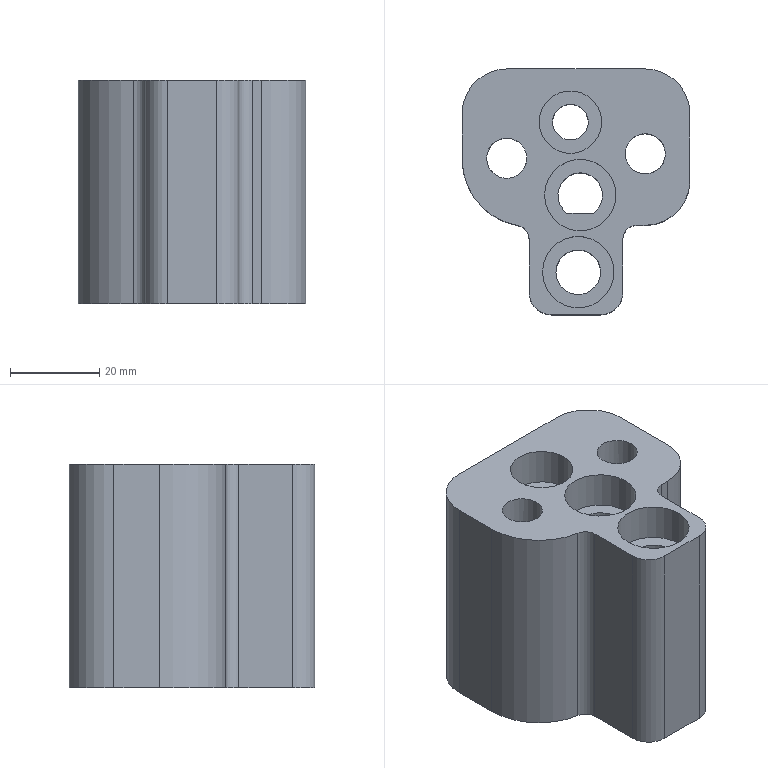Part | STEP file | PN_0023_id1002_x_t | 1 solid | 33 faces | box 51 x 55 x 50 mm | volume 79567 mm3 | cylinder 18 | plane 15 | commonest cylinder face diameters 10 x4 14 x3 20 x3 6 x2 9 x2 16 x2
STEP:
#1=CARTESIAN_POINT('',(276.,20.,95.));
#2=VERTEX_POINT('',#1);
#3=CARTESIAN_POINT('',(276.,8.,95.));
#4=VERTEX_POINT('',#3);
#5=CARTESIAN_POINT('',(276.,28.807,95.));
#6=DIRECTION('',(0.,-1.,0.));
#7=VECTOR('',#6,1.);
#8=LINE('',#5,#7);
#9=EDGE_CURVE('',#2,#4,#8,.T.);
#10=ORIENTED_EDGE('',*,*,#9,.T.);
#11=CARTESIAN_POINT('',(276.,8.,45.));
#12=VERTEX_POINT('',#11);
#13=CARTESIAN_POINT('',(276.,8.,95.));
#14=DIRECTION('',(0.,0.,-1.));
#15=VECTOR('',#14,1.);
#16=LINE('',#13,#15);
#17=EDGE_CURVE('',#4,#12,#16,.T.);
#18=ORIENTED_EDGE('',*,*,#17,.T.);
#19=CARTESIAN_POINT('',(276.,20.,45.));
#20=VERTEX_POINT('',#19);
#21=CARTESIAN_POINT('',(276.,28.807,45.));
#22=DIRECTION('',(0.,1.,0.));
#23=VECTOR('',#22,1.);
#24=LINE('',#21,#23);
#25=EDGE_CURVE('',#12,#20,#24,.T.);
#26=ORIENTED_EDGE('',*,*,#25,.T.);
#27=CARTESIAN_POINT('',(276.,20.,95.));
#28=DIRECTION('',(0.,0.,1.));
#29=VECTOR('',#28,1.);
#30=LINE('',#27,#29);
#31=EDGE_CURVE('',#20,#2,#30,.T.);
#32=ORIENTED_EDGE('',*,*,#31,.T.);
#33=EDGE_LOOP('',(#10,#18,#26,#32));
#34=FACE_OUTER_BOUND('',#33,.T.);
#35=CARTESIAN_POINT('',(276.,28.807,95.));
#36=DIRECTION('',(1.,0.,0.));
#37=DIRECTION('',(0.,0.,-1.));
#38=AXIS2_PLACEMENT_3D('',#35,#36,#37);
#39=PLANE('',#38);
#40=ADVANCED_FACE('',(#34),#39,.T.);
#41=CARTESIAN_POINT('',(255.,20.,45.));
#42=VERTEX_POINT('',#41);
#43=CARTESIAN_POINT('',(255.,8.,45.));
#44=VERTEX_POINT('',#43);
#45=CARTESIAN_POINT('',(255.,28.807,45.));
#46=DIRECTION('',(0.,-1.,0.));
#47=VECTOR('',#46,1.);
#48=LINE('',#45,#47);
#49=EDGE_CURVE('',#42,#44,#48,.T.);
#50=ORIENTED_EDGE('',*,*,#49,.T.);
#51=CARTESIAN_POINT('',(255.,8.,95.));
#52=VERTEX_POINT('',#51);
#53=CARTESIAN_POINT('',(255.,8.,95.));
#54=DIRECTION('',(0.,0.,1.));
#55=VECTOR('',#54,1.);
#56=LINE('',#53,#55);
#57=EDGE_CURVE('',#44,#52,#56,.T.);
#58=ORIENTED_EDGE('',*,*,#57,.T.);
#59=CARTESIAN_POINT('',(255.,20.,95.));
#60=VERTEX_POINT('',#59);
#61=CARTESIAN_POINT('',(255.,28.807,95.));
#62=DIRECTION('',(0.,1.,0.));
#63=VECTOR('',#62,1.);
#64=LINE('',#61,#63);
#65=EDGE_CURVE('',#52,#60,#64,.T.);
#66=ORIENTED_EDGE('',*,*,#65,.T.);
#67=CARTESIAN_POINT('',(255.,20.,95.));
#68=DIRECTION('',(0.,0.,-1.));
#69=VECTOR('',#68,1.);
#70=LINE('',#67,#69);
#71=EDGE_CURVE('',#60,#42,#70,.T.);
#72=ORIENTED_EDGE('',*,*,#71,.T.);
#73=EDGE_LOOP('',(#50,#58,#66,#72));
#74=FACE_OUTER_BOUND('',#73,.T.);
#75=CARTESIAN_POINT('',(255.,28.807,95.));
#76=DIRECTION('',(-1.,0.,0.));
#77=DIRECTION('',(0.,0.,1.));
#78=AXIS2_PLACEMENT_3D('',#75,#76,#77);
#79=PLANE('',#78);
#80=ADVANCED_FACE('',(#74),#79,.T.);
#81=CARTESIAN_POINT('',(263.45,25.762,45.));
#82=VERTEX_POINT('',#81);
#83=CARTESIAN_POINT('',(269.45,25.762,45.));
#84=VERTEX_POINT('',#83);
#85=CARTESIAN_POINT('',(266.45,25.762,45.));
#86=DIRECTION('',(1.,0.,0.));
#87=VECTOR('',#86,1.);
#88=LINE('',#85,#87);
#89=EDGE_CURVE('',#82,#84,#88,.T.);
#90=ORIENTED_EDGE('',*,*,#89,.T.);
#91=CARTESIAN_POINT('',(266.45,29.762,45.));
#92=DIRECTION('',(0.,0.,1.));
#93=DIRECTION('',(1.,0.,0.));
#94=AXIS2_PLACEMENT_3D('',#91,#92,#93);
#95=CIRCLE('',#94,5.);
#96=EDGE_CURVE('',#84,#82,#95,.T.);
#97=ORIENTED_EDGE('',*,*,#96,.T.);
#98=EDGE_LOOP('',(#90,#97));
#99=FACE_BOUND('',#98,.T.);
#100=CARTESIAN_POINT('',(271.,12.5,45.));
#101=VERTEX_POINT('',#100);
#102=CARTESIAN_POINT('',(266.,12.5,45.));
#103=DIRECTION('',(0.,0.,1.));
#104=DIRECTION('',(1.,0.,0.));
#105=AXIS2_PLACEMENT_3D('',#102,#103,#104);
#106=CIRCLE('',#105,5.);
#107=EDGE_CURVE('',#101,#101,#106,.T.);
#108=ORIENTED_EDGE('',*,*,#107,.T.);
#109=EDGE_LOOP('',(#108));
#110=FACE_BOUND('',#109,.T.);
#111=CARTESIAN_POINT('',(268.25,46.114,45.));
#112=VERTEX_POINT('',#111);
#113=CARTESIAN_POINT('',(264.25,46.114,45.));
#114=DIRECTION('',(0.,0.,1.));
#115=DIRECTION('',(1.,0.,0.));
#116=AXIS2_PLACEMENT_3D('',#113,#114,#115);
#117=CIRCLE('',#116,4.);
#118=EDGE_CURVE('',#112,#112,#117,.T.);
#119=ORIENTED_EDGE('',*,*,#118,.T.);
#120=EDGE_LOOP('',(#119));
#121=FACE_BOUND('',#120,.T.);
#122=CARTESIAN_POINT('',(281.,46.,45.));
#123=VERTEX_POINT('',#122);
#124=CARTESIAN_POINT('',(281.,39.,45.));
#125=DIRECTION('',(0.,0.,1.));
#126=DIRECTION('',(0.,1.,0.));
#127=AXIS2_PLACEMENT_3D('',#124,#125,#126);
#128=CIRCLE('',#127,7.);
#129=EDGE_CURVE('',#123,#123,#128,.T.);
#130=ORIENTED_EDGE('',*,*,#129,.T.);
#131=EDGE_LOOP('',(#130));
#132=FACE_BOUND('',#131,.T.);
#133=CARTESIAN_POINT('',(250.,31.,45.));
#134=VERTEX_POINT('',#133);
#135=CARTESIAN_POINT('',(250.,38.,45.));
#136=DIRECTION('',(0.,0.,1.));
#137=DIRECTION('',(0.,-1.,0.));
#138=AXIS2_PLACEMENT_3D('',#135,#136,#137);
#139=CIRCLE('',#138,7.);
#140=EDGE_CURVE('',#134,#134,#139,.T.);
#141=ORIENTED_EDGE('',*,*,#140,.T.);
#142=EDGE_LOOP('',(#141));
#143=FACE_BOUND('',#142,.T.);
#144=CARTESIAN_POINT('',(252.5,22.958,45.));
#145=VERTEX_POINT('',#144);
#146=CARTESIAN_POINT('',(252.,20.,45.));
#147=DIRECTION('',(0.,0.,1.));
#148=DIRECTION('',(1.,0.,0.));
#149=AXIS2_PLACEMENT_3D('',#146,#147,#148);
#150=CIRCLE('',#149,3.);
#151=EDGE_CURVE('',#42,#145,#150,.T.);
#152=ORIENTED_EDGE('',*,*,#151,.T.);
#153=CARTESIAN_POINT('',(240.,37.748,45.));
#154=VERTEX_POINT('',#153);
#155=CARTESIAN_POINT('',(255.,37.748,45.));
#156=DIRECTION('',(0.,0.,-1.));
#157=DIRECTION('',(1.,0.,0.));
#158=AXIS2_PLACEMENT_3D('',#155,#156,#157);
#159=CIRCLE('',#158,15.);
#160=EDGE_CURVE('',#145,#154,#159,.T.);
#161=ORIENTED_EDGE('',*,*,#160,.T.);
#162=CARTESIAN_POINT('',(240.,48.,45.));
#163=VERTEX_POINT('',#162);
#164=CARTESIAN_POINT('',(240.,28.807,45.));
#165=DIRECTION('',(0.,-1.,0.));
#166=VECTOR('',#165,1.);
#167=LINE('',#164,#166);
#168=EDGE_CURVE('',#163,#154,#167,.T.);
#169=ORIENTED_EDGE('',*,*,#168,.F.);
#170=CARTESIAN_POINT('',(250.,58.,45.));
#171=VERTEX_POINT('',#170);
#172=CARTESIAN_POINT('',(250.,48.,45.));
#173=DIRECTION('',(0.,0.,-1.));
#174=DIRECTION('',(1.,0.,0.));
#175=AXIS2_PLACEMENT_3D('',#172,#173,#174);
#176=CIRCLE('',#175,10.);
#177=EDGE_CURVE('',#163,#171,#176,.T.);
#178=ORIENTED_EDGE('',*,*,#177,.T.);
#179=CARTESIAN_POINT('',(281.,58.,45.));
#180=VERTEX_POINT('',#179);
#181=CARTESIAN_POINT('',(265.85,58.,45.));
#182=DIRECTION('',(-1.,0.,0.));
#183=VECTOR('',#182,1.);
#184=LINE('',#181,#183);
#185=EDGE_CURVE('',#180,#171,#184,.T.);
#186=ORIENTED_EDGE('',*,*,#185,.F.);
#187=CARTESIAN_POINT('',(291.,48.,45.));
#188=VERTEX_POINT('',#187);
#189=CARTESIAN_POINT('',(281.,48.,45.));
#190=DIRECTION('',(0.,0.,-1.));
#191=DIRECTION('',(1.,0.,0.));
#192=AXIS2_PLACEMENT_3D('',#189,#190,#191);
#193=CIRCLE('',#192,10.);
#194=EDGE_CURVE('',#180,#188,#193,.T.);
#195=ORIENTED_EDGE('',*,*,#194,.T.);
#196=CARTESIAN_POINT('',(291.,33.,45.));
#197=VERTEX_POINT('',#196);
#198=CARTESIAN_POINT('',(291.,58.,45.));
#199=DIRECTION('',(0.,-1.,0.));
#200=VECTOR('',#199,1.);
#201=LINE('',#198,#200);
#202=EDGE_CURVE('',#188,#197,#201,.T.);
#203=ORIENTED_EDGE('',*,*,#202,.T.);
#204=CARTESIAN_POINT('',(281.,23.,45.));
#205=VERTEX_POINT('',#204);
#206=CARTESIAN_POINT('',(281.,33.,45.));
#207=DIRECTION('',(0.,0.,-1.));
#208=DIRECTION('',(1.,0.,0.));
#209=AXIS2_PLACEMENT_3D('',#206,#207,#208);
#210=CIRCLE('',#209,10.);
#211=EDGE_CURVE('',#197,#205,#210,.T.);
#212=ORIENTED_EDGE('',*,*,#211,.T.);
#213=CARTESIAN_POINT('',(279.,23.,45.));
#214=VERTEX_POINT('',#213);
#215=CARTESIAN_POINT('',(265.85,23.,45.));
#216=DIRECTION('',(-1.,0.,0.));
#217=VECTOR('',#216,1.);
#218=LINE('',#215,#217);
#219=EDGE_CURVE('',#205,#214,#218,.T.);
#220=ORIENTED_EDGE('',*,*,#219,.T.);
#221=CARTESIAN_POINT('',(279.,20.,45.));
#222=DIRECTION('',(0.,0.,1.));
#223=DIRECTION('',(1.,0.,0.));
#224=AXIS2_PLACEMENT_3D('',#221,#222,#223);
#225=CIRCLE('',#224,3.);
#226=EDGE_CURVE('',#214,#20,#225,.T.);
#227=ORIENTED_EDGE('',*,*,#226,.T.);
#228=ORIENTED_EDGE('',*,*,#25,.F.);
#229=CARTESIAN_POINT('',(271.,3.,45.));
#230=VERTEX_POINT('',#229);
#231=CARTESIAN_POINT('',(271.,8.,45.));
#232=DIRECTION('',(0.,0.,-1.));
#233=DIRECTION('',(1.,0.,0.));
#234=AXIS2_PLACEMENT_3D('',#231,#232,#233);
#235=CIRCLE('',#234,5.);
#236=EDGE_CURVE('',#12,#230,#235,.T.);
#237=ORIENTED_EDGE('',*,*,#236,.T.);
#238=CARTESIAN_POINT('',(260.,3.,45.));
#239=VERTEX_POINT('',#238);
#240=CARTESIAN_POINT('',(265.85,3.,45.));
#241=DIRECTION('',(1.,0.,0.));
#242=VECTOR('',#241,1.);
#243=LINE('',#240,#242);
#244=EDGE_CURVE('',#239,#230,#243,.T.);
#245=ORIENTED_EDGE('',*,*,#244,.F.);
#246=CARTESIAN_POINT('',(260.,8.,45.));
#247=DIRECTION('',(0.,0.,-1.));
#248=DIRECTION('',(1.,0.,0.));
#249=AXIS2_PLACEMENT_3D('',#246,#247,#248);
#250=CIRCLE('',#249,5.);
#251=EDGE_CURVE('',#239,#44,#250,.T.);
#252=ORIENTED_EDGE('',*,*,#251,.T.);
#253=ORIENTED_EDGE('',*,*,#49,.F.);
#254=EDGE_LOOP('',(#152,#161,#169,#178,#186,#195,#203,#212,#220,#227,#228,#237,#245,#252,#253));
#255=FACE_BOUND('',#254,.T.);
#256=CARTESIAN_POINT('',(265.85,28.807,45.));
#257=DIRECTION('',(0.,0.,1.));
#258=DIRECTION('',(1.,0.,0.));
#259=AXIS2_PLACEMENT_3D('',#256,#257,#258);
#260=PLANE('',#259);
#261=ADVANCED_FACE('',(#99,#110,#121,#132,#143,#255),#260,.F.);
#262=ORIENTED_EDGE('',*,*,#244,.T.);
#263=CARTESIAN_POINT('',(271.,3.,95.));
#264=VERTEX_POINT('',#263);
#265=CARTESIAN_POINT('',(271.,3.,95.));
#266=DIRECTION('',(0.,0.,1.));
#267=VECTOR('',#266,1.);
#268=LINE('',#265,#267);
#269=EDGE_CURVE('',#230,#264,#268,.T.);
#270=ORIENTED_EDGE('',*,*,#269,.T.);
#271=CARTESIAN_POINT('',(260.,3.,95.));
#272=VERTEX_POINT('',#271);
#273=CARTESIAN_POINT('',(265.85,3.,95.));
#274=DIRECTION('',(-1.,0.,0.));
#275=VECTOR('',#274,1.);
#276=LINE('',#273,#275);
#277=EDGE_CURVE('',#264,#272,#276,.T.);
#278=ORIENTED_EDGE('',*,*,#277,.T.);
#279=CARTESIAN_POINT('',(260.,3.,95.));
#280=DIRECTION('',(0.,0.,-1.));
#281=VECTOR('',#280,1.);
#282=LINE('',#279,#281);
#283=EDGE_CURVE('',#272,#239,#282,.T.);
#284=ORIENTED_EDGE('',*,*,#283,.T.);
#285=EDGE_LOOP('',(#262,#270,#278,#284));
#286=FACE_OUTER_BOUND('',#285,.T.);
#287=CARTESIAN_POINT('',(265.85,3.,95.));
#288=DIRECTION('',(0.,-1.,0.));
#289=DIRECTION('',(0.,0.,-1.));
#290=AXIS2_PLACEMENT_3D('',#287,#288,#289);
#291=PLANE('',#290);
#292=ADVANCED_FACE('',(#286),#291,.T.);
#293=ORIENTED_EDGE('',*,*,#185,.T.);
#294=CARTESIAN_POINT('',(250.,58.,95.));
#295=VERTEX_POINT('',#294);
#296=CARTESIAN_POINT('',(250.,58.,95.));
#297=DIRECTION('',(0.,0.,1.));
#298=VECTOR('',#297,1.);
#299=LINE('',#296,#298);
#300=EDGE_CURVE('',#171,#295,#299,.T.);
#301=ORIENTED_EDGE('',*,*,#300,.T.);
#302=CARTESIAN_POINT('',(281.,58.,95.));
#303=VERTEX_POINT('',#302);
#304=CARTESIAN_POINT('',(265.85,58.,95.));
#305=DIRECTION('',(1.,0.,0.));
#306=VECTOR('',#305,1.);
#307=LINE('',#304,#306);
#308=EDGE_CURVE('',#295,#303,#307,.T.);
#309=ORIENTED_EDGE('',*,*,#308,.T.);
#310=CARTESIAN_POINT('',(281.,58.,45.));
#311=DIRECTION('',(0.,0.,-1.));
#312=VECTOR('',#311,1.);
#313=LINE('',#310,#312);
#314=EDGE_CURVE('',#303,#180,#313,.T.);
#315=ORIENTED_EDGE('',*,*,#314,.T.);
#316=EDGE_LOOP('',(#293,#301,#309,#315));
#317=FACE_OUTER_BOUND('',#316,.T.);
#318=CARTESIAN_POINT('',(265.85,58.,95.));
#319=DIRECTION('',(0.,1.,0.));
#320=DIRECTION('',(0.,0.,1.));
#321=AXIS2_PLACEMENT_3D('',#318,#319,#320);
#322=PLANE('',#321);
#323=ADVANCED_FACE('',(#317),#322,.T.);
#324=CARTESIAN_POINT('',(274.45,29.762,95.));
#325=VERTEX_POINT('',#324);
#326=CARTESIAN_POINT('',(266.45,29.762,95.));
#327=DIRECTION('',(0.,0.,-1.));
#328=DIRECTION('',(1.,0.,0.));
#329=AXIS2_PLACEMENT_3D('',#326,#327,#328);
#330=CIRCLE('',#329,8.);
#331=EDGE_CURVE('',#325,#325,#330,.T.);
#332=ORIENTED_EDGE('',*,*,#331,.T.);
#333=EDGE_LOOP('',(#332));
#334=FACE_BOUND('',#333,.T.);
#335=CARTESIAN_POINT('',(274.,12.5,95.));
#336=VERTEX_POINT('',#335);
#337=CARTESIAN_POINT('',(266.,12.5,95.));
#338=DIRECTION('',(0.,0.,-1.));
#339=DIRECTION('',(1.,0.,0.));
#340=AXIS2_PLACEMENT_3D('',#337,#338,#339);
#341=CIRCLE('',#340,8.);
#342=EDGE_CURVE('',#336,#336,#341,.T.);
#343=ORIENTED_EDGE('',*,*,#342,.T.);
#344=EDGE_LOOP('',(#343));
#345=FACE_BOUND('',#344,.T.);
#346=CARTESIAN_POINT('',(271.25,46.114,95.));
#347=VERTEX_POINT('',#346);
#348=CARTESIAN_POINT('',(264.25,46.114,95.));
#349=DIRECTION('',(0.,0.,-1.));
#350=DIRECTION('',(1.,0.,0.));
#351=AXIS2_PLACEMENT_3D('',#348,#349,#350);
#352=CIRCLE('',#351,7.);
#353=EDGE_CURVE('',#347,#347,#352,.T.);
#354=ORIENTED_EDGE('',*,*,#353,.T.);
#355=EDGE_LOOP('',(#354));
#356=FACE_BOUND('',#355,.T.);
#357=CARTESIAN_POINT('',(285.5,39.,95.));
#358=VERTEX_POINT('',#357);
#359=CARTESIAN_POINT('',(281.,39.,95.));
#360=DIRECTION('',(0.,0.,1.));
#361=DIRECTION('',(1.,0.,0.));
#362=AXIS2_PLACEMENT_3D('',#359,#360,#361);
#363=CIRCLE('',#362,4.5);
#364=EDGE_CURVE('',#358,#358,#363,.T.);
#365=ORIENTED_EDGE('',*,*,#364,.F.);
#366=EDGE_LOOP('',(#365));
#367=FACE_BOUND('',#366,.T.);
#368=CARTESIAN_POINT('',(254.5,38.,95.));
#369=VERTEX_POINT('',#368);
#370=CARTESIAN_POINT('',(250.,38.,95.));
#371=DIRECTION('',(0.,0.,1.));
#372=DIRECTION('',(1.,0.,0.));
#373=AXIS2_PLACEMENT_3D('',#370,#371,#372);
#374=CIRCLE('',#373,4.5);
#375=EDGE_CURVE('',#369,#369,#374,.T.);
#376=ORIENTED_EDGE('',*,*,#375,.F.);
#377=EDGE_LOOP('',(#376));
#378=FACE_BOUND('',#377,.T.);
#379=CARTESIAN_POINT('',(240.,48.,95.));
#380=VERTEX_POINT('',#379);
#381=CARTESIAN_POINT('',(240.,37.748,95.));
#382=VERTEX_POINT('',#381);
#383=CARTESIAN_POINT('',(240.,58.,95.));
#384=DIRECTION('',(0.,-1.,0.));
#385=VECTOR('',#384,1.);
#386=LINE('',#383,#385);
#387=EDGE_CURVE('',#380,#382,#386,.T.);
#388=ORIENTED_EDGE('',*,*,#387,.T.);
#389=CARTESIAN_POINT('',(252.5,22.958,95.));
#390=VERTEX_POINT('',#389);
#391=CARTESIAN_POINT('',(255.,37.748,95.));
#392=DIRECTION('',(0.,0.,1.));
#393=DIRECTION('',(1.,0.,0.));
#394=AXIS2_PLACEMENT_3D('',#391,#392,#393);
#395=CIRCLE('',#394,15.);
#396=EDGE_CURVE('',#382,#390,#395,.T.);
#397=ORIENTED_EDGE('',*,*,#396,.T.);
#398=CARTESIAN_POINT('',(252.,20.,95.));
#399=DIRECTION('',(0.,0.,-1.));
#400=DIRECTION('',(1.,0.,0.));
#401=AXIS2_PLACEMENT_3D('',#398,#399,#400);
#402=CIRCLE('',#401,3.);
#403=EDGE_CURVE('',#390,#60,#402,.T.);
#404=ORIENTED_EDGE('',*,*,#403,.T.);
#405=ORIENTED_EDGE('',*,*,#65,.F.);
#406=CARTESIAN_POINT('',(260.,8.,95.));
#407=DIRECTION('',(0.,0.,1.));
#408=DIRECTION('',(1.,0.,0.));
#409=AXIS2_PLACEMENT_3D('',#406,#407,#408);
#410=CIRCLE('',#409,5.);
#411=EDGE_CURVE('',#52,#272,#410,.T.);
#412=ORIENTED_EDGE('',*,*,#411,.T.);
#413=ORIENTED_EDGE('',*,*,#277,.F.);
#414=CARTESIAN_POINT('',(271.,8.,95.));
#415=DIRECTION('',(0.,0.,1.));
#416=DIRECTION('',(1.,0.,0.));
#417=AXIS2_PLACEMENT_3D('',#414,#415,#416);
#418=CIRCLE('',#417,5.);
#419=EDGE_CURVE('',#264,#4,#418,.T.);
#420=ORIENTED_EDGE('',*,*,#419,.T.);
#421=ORIENTED_EDGE('',*,*,#9,.F.);
#422=CARTESIAN_POINT('',(279.,23.,95.));
#423=VERTEX_POINT('',#422);
#424=CARTESIAN_POINT('',(279.,20.,95.));
#425=DIRECTION('',(0.,0.,-1.));
#426=DIRECTION('',(1.,0.,0.));
#427=AXIS2_PLACEMENT_3D('',#424,#425,#426);
#428=CIRCLE('',#427,3.);
#429=EDGE_CURVE('',#2,#423,#428,.T.);
#430=ORIENTED_EDGE('',*,*,#429,.T.);
#431=CARTESIAN_POINT('',(281.,23.,95.));
#432=VERTEX_POINT('',#431);
#433=CARTESIAN_POINT('',(265.85,23.,95.));
#434=DIRECTION('',(1.,0.,0.));
#435=VECTOR('',#434,1.);
#436=LINE('',#433,#435);
#437=EDGE_CURVE('',#423,#432,#436,.T.);
#438=ORIENTED_EDGE('',*,*,#437,.T.);
#439=CARTESIAN_POINT('',(291.,33.,95.));
#440=VERTEX_POINT('',#439);
#441=CARTESIAN_POINT('',(281.,33.,95.));
#442=DIRECTION('',(0.,0.,1.));
#443=DIRECTION('',(1.,0.,0.));
#444=AXIS2_PLACEMENT_3D('',#441,#442,#443);
#445=CIRCLE('',#444,10.);
#446=EDGE_CURVE('',#432,#440,#445,.T.);
#447=ORIENTED_EDGE('',*,*,#446,.T.);
#448=CARTESIAN_POINT('',(291.,48.,95.));
#449=VERTEX_POINT('',#448);
#450=CARTESIAN_POINT('',(291.,28.807,95.));
#451=DIRECTION('',(0.,-1.,0.));
#452=VECTOR('',#451,1.);
#453=LINE('',#450,#452);
#454=EDGE_CURVE('',#449,#440,#453,.T.);
#455=ORIENTED_EDGE('',*,*,#454,.F.);
#456=CARTESIAN_POINT('',(281.,48.,95.));
#457=DIRECTION('',(0.,0.,1.));
#458=DIRECTION('',(1.,0.,0.));
#459=AXIS2_PLACEMENT_3D('',#456,#457,#458);
#460=CIRCLE('',#459,10.);
#461=EDGE_CURVE('',#449,#303,#460,.T.);
#462=ORIENTED_EDGE('',*,*,#461,.T.);
#463=ORIENTED_EDGE('',*,*,#308,.F.);
#464=CARTESIAN_POINT('',(250.,48.,95.));
#465=DIRECTION('',(0.,0.,1.));
#466=DIRECTION('',(1.,0.,0.));
#467=AXIS2_PLACEMENT_3D('',#464,#465,#466);
#468=CIRCLE('',#467,10.);
#469=EDGE_CURVE('',#295,#380,#468,.T.);
#470=ORIENTED_EDGE('',*,*,#469,.T.);
#471=EDGE_LOOP('',(#388,#397,#404,#405,#412,#413,#420,#421,#430,#438,#447,#455,#462,#463,#470));
#472=FACE_BOUND('',#471,.T.);
#473=CARTESIAN_POINT('',(265.85,28.807,95.));
#474=DIRECTION('',(0.,0.,1.));
#475=DIRECTION('',(1.,0.,0.));
#476=AXIS2_PLACEMENT_3D('',#473,#474,#475);
#477=PLANE('',#476);
#478=ADVANCED_FACE('',(#334,#345,#356,#367,#378,#472),#477,.T.);
#479=ORIENTED_EDGE('',*,*,#168,.T.);
#480=CARTESIAN_POINT('',(240.,37.748,95.));
#481=DIRECTION('',(0.,0.,1.));
#482=VECTOR('',#481,1.);
#483=LINE('',#480,#482);
#484=EDGE_CURVE('',#154,#382,#483,.T.);
#485=ORIENTED_EDGE('',*,*,#484,.T.);
#486=ORIENTED_EDGE('',*,*,#387,.F.);
#487=CARTESIAN_POINT('',(240.,48.,45.));
#488=DIRECTION('',(0.,0.,-1.));
#489=VECTOR('',#488,1.);
#490=LINE('',#487,#489);
#491=EDGE_CURVE('',#380,#163,#490,.T.);
#492=ORIENTED_EDGE('',*,*,#491,.T.);
#493=EDGE_LOOP('',(#479,#485,#486,#492));
#494=FACE_OUTER_BOUND('',#493,.T.);
#495=CARTESIAN_POINT('',(240.,58.,95.));
#496=DIRECTION('',(1.,0.,0.));
#497=DIRECTION('',(0.,0.,-1.));
#498=AXIS2_PLACEMENT_3D('',#495,#496,#497);
#499=PLANE('',#498);
#500=ADVANCED_FACE('',(#494),#499,.F.);
#501=ORIENTED_EDGE('',*,*,#219,.F.);
#502=CARTESIAN_POINT('',(281.,23.,95.));
#503=DIRECTION('',(0.,0.,1.));
#504=VECTOR('',#503,1.);
#505=LINE('',#502,#504);
#506=EDGE_CURVE('',#205,#432,#505,.T.);
#507=ORIENTED_EDGE('',*,*,#506,.T.);
#508=ORIENTED_EDGE('',*,*,#437,.F.);
#509=CARTESIAN_POINT('',(279.,23.,95.));
#510=DIRECTION('',(0.,0.,-1.));
#511=VECTOR('',#510,1.);
#512=LINE('',#509,#511);
#513=EDGE_CURVE('',#423,#214,#512,.T.);
#514=ORIENTED_EDGE('',*,*,#513,.T.);
#515=EDGE_LOOP('',(#501,#507,#508,#514));
#516=FACE_OUTER_BOUND('',#515,.T.);
#517=CARTESIAN_POINT('',(265.85,23.,95.));
#518=DIRECTION('',(0.,1.,0.));
#519=DIRECTION('',(0.,0.,1.));
#520=AXIS2_PLACEMENT_3D('',#517,#518,#519);
#521=PLANE('',#520);
#522=ADVANCED_FACE('',(#516),#521,.F.);
#523=ORIENTED_EDGE('',*,*,#454,.T.);
#524=CARTESIAN_POINT('',(291.,33.,95.));
#525=DIRECTION('',(0.,0.,-1.));
#526=VECTOR('',#525,1.);
#527=LINE('',#524,#526);
#528=EDGE_CURVE('',#440,#197,#527,.T.);
#529=ORIENTED_EDGE('',*,*,#528,.T.);
#530=ORIENTED_EDGE('',*,*,#202,.F.);
#531=CARTESIAN_POINT('',(291.,48.,95.));
#532=DIRECTION('',(0.,0.,1.));
#533=VECTOR('',#532,1.);
#534=LINE('',#531,#533);
#535=EDGE_CURVE('',#188,#449,#534,.T.);
#536=ORIENTED_EDGE('',*,*,#535,.T.);
#537=EDGE_LOOP('',(#523,#529,#530,#536));
#538=FACE_OUTER_BOUND('',#537,.T.);
#539=CARTESIAN_POINT('',(291.,58.,95.));
#540=DIRECTION('',(1.,0.,0.));
#541=DIRECTION('',(0.,0.,-1.));
#542=AXIS2_PLACEMENT_3D('',#539,#540,#541);
#543=PLANE('',#542);
#544=ADVANCED_FACE('',(#538),#543,.T.);
#545=ORIENTED_EDGE('',*,*,#226,.F.);
#546=ORIENTED_EDGE('',*,*,#513,.F.);
#547=ORIENTED_EDGE('',*,*,#429,.F.);
#548=ORIENTED_EDGE('',*,*,#31,.F.);
#549=EDGE_LOOP('',(#545,#546,#547,#548));
#550=FACE_OUTER_BOUND('',#549,.T.);
#551=CARTESIAN_POINT('',(279.,20.,95.));
#552=DIRECTION('',(0.,0.,1.));
#553=DIRECTION('',(1.,0.,0.));
#554=AXIS2_PLACEMENT_3D('',#551,#552,#553);
#555=CYLINDRICAL_SURFACE('',#554,3.);
#556=ADVANCED_FACE('',(#550),#555,.F.);
#557=ORIENTED_EDGE('',*,*,#403,.F.);
#558=CARTESIAN_POINT('',(252.5,22.958,70.));
#559=DIRECTION('',(0.,0.,-1.));
#560=VECTOR('',#559,1.);
#561=LINE('',#558,#560);
#562=EDGE_CURVE('',#390,#145,#561,.T.);
#563=ORIENTED_EDGE('',*,*,#562,.T.);
#564=ORIENTED_EDGE('',*,*,#151,.F.);
#565=ORIENTED_EDGE('',*,*,#71,.F.);
#566=EDGE_LOOP('',(#557,#563,#564,#565));
#567=FACE_OUTER_BOUND('',#566,.T.);
#568=CARTESIAN_POINT('',(252.,20.,95.));
#569=DIRECTION('',(0.,0.,-1.));
#570=DIRECTION('',(-1.,0.,0.));
#571=AXIS2_PLACEMENT_3D('',#568,#569,#570);
#572=CYLINDRICAL_SURFACE('',#571,3.);
#573=ADVANCED_FACE('',(#567),#572,.F.);
#574=ORIENTED_EDGE('',*,*,#446,.F.);
#575=ORIENTED_EDGE('',*,*,#506,.F.);
#576=ORIENTED_EDGE('',*,*,#211,.F.);
#577=ORIENTED_EDGE('',*,*,#528,.F.);
#578=EDGE_LOOP('',(#574,#575,#576,#577));
#579=FACE_OUTER_BOUND('',#578,.T.);
#580=CARTESIAN_POINT('',(281.,33.,95.));
#581=DIRECTION('',(0.,0.,1.));
#582=DIRECTION('',(1.,0.,0.));
#583=AXIS2_PLACEMENT_3D('',#580,#581,#582);
#584=CYLINDRICAL_SURFACE('',#583,10.);
#585=ADVANCED_FACE('',(#579),#584,.T.);
#586=ORIENTED_EDGE('',*,*,#469,.F.);
#587=ORIENTED_EDGE('',*,*,#300,.F.);
#588=ORIENTED_EDGE('',*,*,#177,.F.);
#589=ORIENTED_EDGE('',*,*,#491,.F.);
#590=EDGE_LOOP('',(#586,#587,#588,#589));
#591=FACE_OUTER_BOUND('',#590,.T.);
#592=CARTESIAN_POINT('',(250.,48.,95.));
#593=DIRECTION('',(0.,0.,1.));
#594=DIRECTION('',(1.,0.,0.));
#595=AXIS2_PLACEMENT_3D('',#592,#593,#594);
#596=CYLINDRICAL_SURFACE('',#595,10.);
#597=ADVANCED_FACE('',(#591),#596,.T.);
#598=ORIENTED_EDGE('',*,*,#461,.F.);
#599=ORIENTED_EDGE('',*,*,#535,.F.);
#600=ORIENTED_EDGE('',*,*,#194,.F.);
#601=ORIENTED_EDGE('',*,*,#314,.F.);
#602=EDGE_LOOP('',(#598,#599,#600,#601));
#603=FACE_OUTER_BOUND('',#602,.T.);
#604=CARTESIAN_POINT('',(281.,48.,95.));
#605=DIRECTION('',(0.,0.,-1.));
#606=DIRECTION('',(-1.,0.,0.));
#607=AXIS2_PLACEMENT_3D('',#604,#605,#606);
#608=CYLINDRICAL_SURFACE('',#607,10.);
#609=ADVANCED_FACE('',(#603),#608,.T.);
#610=ORIENTED_EDGE('',*,*,#419,.F.);
#611=ORIENTED_EDGE('',*,*,#269,.F.);
#612=ORIENTED_EDGE('',*,*,#236,.F.);
#613=ORIENTED_EDGE('',*,*,#17,.F.);
#614=EDGE_LOOP('',(#610,#611,#612,#613));
#615=FACE_OUTER_BOUND('',#614,.T.);
#616=CARTESIAN_POINT('',(271.,8.,95.));
#617=DIRECTION('',(0.,0.,-1.));
#618=DIRECTION('',(-1.,0.,0.));
#619=AXIS2_PLACEMENT_3D('',#616,#617,#618);
#620=CYLINDRICAL_SURFACE('',#619,5.);
#621=ADVANCED_FACE('',(#615),#620,.T.);
#622=ORIENTED_EDGE('',*,*,#411,.F.);
#623=ORIENTED_EDGE('',*,*,#57,.F.);
#624=ORIENTED_EDGE('',*,*,#251,.F.);
#625=ORIENTED_EDGE('',*,*,#283,.F.);
#626=EDGE_LOOP('',(#622,#623,#624,#625));
#627=FACE_OUTER_BOUND('',#626,.T.);
#628=CARTESIAN_POINT('',(260.,8.,95.));
#629=DIRECTION('',(0.,0.,-1.));
#630=DIRECTION('',(-1.,0.,0.));
#631=AXIS2_PLACEMENT_3D('',#628,#629,#630);
#632=CYLINDRICAL_SURFACE('',#631,5.);
#633=ADVANCED_FACE('',(#627),#632,.T.);
#634=ORIENTED_EDGE('',*,*,#396,.F.);
#635=ORIENTED_EDGE('',*,*,#484,.F.);
#636=ORIENTED_EDGE('',*,*,#160,.F.);
#637=ORIENTED_EDGE('',*,*,#562,.F.);
#638=EDGE_LOOP('',(#634,#635,#636,#637));
#639=FACE_OUTER_BOUND('',#638,.T.);
#640=CARTESIAN_POINT('',(255.,37.748,95.));
#641=DIRECTION('',(0.,0.,-1.));
#642=DIRECTION('',(-1.,0.,0.));
#643=AXIS2_PLACEMENT_3D('',#640,#641,#642);
#644=CYLINDRICAL_SURFACE('',#643,15.);
#645=ADVANCED_FACE('',(#639),#644,.T.);
#646=ORIENTED_EDGE('',*,*,#375,.T.);
#647=EDGE_LOOP('',(#646));
#648=FACE_BOUND('',#647,.T.);
#649=CARTESIAN_POINT('',(250.,33.5,75.));
#650=VERTEX_POINT('',#649);
#651=CARTESIAN_POINT('',(250.,38.,75.));
#652=DIRECTION('',(0.,0.,1.));
#653=DIRECTION('',(0.,-1.,0.));
#654=AXIS2_PLACEMENT_3D('',#651,#652,#653);
#655=CIRCLE('',#654,4.5);
#656=EDGE_CURVE('',#650,#650,#655,.T.);
#657=ORIENTED_EDGE('',*,*,#656,.F.);
#658=EDGE_LOOP('',(#657));
#659=FACE_BOUND('',#658,.T.);
#660=CARTESIAN_POINT('',(250.,38.,105.));
#661=DIRECTION('',(0.,0.,-1.));
#662=DIRECTION('',(0.,1.,0.));
#663=AXIS2_PLACEMENT_3D('',#660,#661,#662);
#664=CYLINDRICAL_SURFACE('',#663,4.5);
#665=ADVANCED_FACE('',(#648,#659),#664,.F.);
#666=ORIENTED_EDGE('',*,*,#656,.T.);
#667=EDGE_LOOP('',(#666));
#668=FACE_BOUND('',#667,.T.);
#669=CARTESIAN_POINT('',(250.,45.,75.));
#670=VERTEX_POINT('',#669);
#671=CARTESIAN_POINT('',(250.,38.,75.));
#672=DIRECTION('',(0.,0.,1.));
#673=DIRECTION('',(0.,1.,0.));
#674=AXIS2_PLACEMENT_3D('',#671,#672,#673);
#675=CIRCLE('',#674,7.);
#676=EDGE_CURVE('',#670,#670,#675,.T.);
#677=ORIENTED_EDGE('',*,*,#676,.F.);
#678=EDGE_LOOP('',(#677));
#679=FACE_BOUND('',#678,.T.);
#680=CARTESIAN_POINT('',(250.,38.,75.));
#681=DIRECTION('',(0.,0.,1.));
#682=DIRECTION('',(0.,-1.,0.));
#683=AXIS2_PLACEMENT_3D('',#680,#681,#682);
#684=PLANE('',#683);
#685=ADVANCED_FACE('',(#668,#679),#684,.F.);
#686=ORIENTED_EDGE('',*,*,#140,.F.);
#687=EDGE_LOOP('',(#686));
#688=FACE_BOUND('',#687,.T.);
#689=ORIENTED_EDGE('',*,*,#676,.T.);
#690=EDGE_LOOP('',(#689));
#691=FACE_BOUND('',#690,.T.);
#692=CARTESIAN_POINT('',(250.,38.,75.));
#693=DIRECTION('',(0.,0.,-1.));
#694=DIRECTION('',(0.,1.,0.));
#695=AXIS2_PLACEMENT_3D('',#692,#693,#694);
#696=CYLINDRICAL_SURFACE('',#695,7.);
#697=ADVANCED_FACE('',(#688,#691),#696,.F.);
#698=ORIENTED_EDGE('',*,*,#364,.T.);
#699=EDGE_LOOP('',(#698));
#700=FACE_BOUND('',#699,.T.);
#701=CARTESIAN_POINT('',(281.,43.5,75.));
#702=VERTEX_POINT('',#701);
#703=CARTESIAN_POINT('',(281.,39.,75.));
#704=DIRECTION('',(0.,0.,1.));
#705=DIRECTION('',(0.,1.,0.));
#706=AXIS2_PLACEMENT_3D('',#703,#704,#705);
#707=CIRCLE('',#706,4.5);
#708=EDGE_CURVE('',#702,#702,#707,.T.);
#709=ORIENTED_EDGE('',*,*,#708,.F.);
#710=EDGE_LOOP('',(#709));
#711=FACE_BOUND('',#710,.T.);
#712=CARTESIAN_POINT('',(281.,39.,105.));
#713=DIRECTION('',(0.,0.,-1.));
#714=DIRECTION('',(0.,-1.,0.));
#715=AXIS2_PLACEMENT_3D('',#712,#713,#714);
#716=CYLINDRICAL_SURFACE('',#715,4.5);
#717=ADVANCED_FACE('',(#700,#711),#716,.F.);
#718=ORIENTED_EDGE('',*,*,#708,.T.);
#719=EDGE_LOOP('',(#718));
#720=FACE_BOUND('',#719,.T.);
#721=CARTESIAN_POINT('',(281.,32.,75.));
#722=VERTEX_POINT('',#721);
#723=CARTESIAN_POINT('',(281.,39.,75.));
#724=DIRECTION('',(0.,0.,1.));
#725=DIRECTION('',(0.,-1.,0.));
#726=AXIS2_PLACEMENT_3D('',#723,#724,#725);
#727=CIRCLE('',#726,7.);
#728=EDGE_CURVE('',#722,#722,#727,.T.);
#729=ORIENTED_EDGE('',*,*,#728,.F.);
#730=EDGE_LOOP('',(#729));
#731=FACE_BOUND('',#730,.T.);
#732=CARTESIAN_POINT('',(281.,39.,75.));
#733=DIRECTION('',(0.,0.,1.));
#734=DIRECTION('',(0.,1.,0.));
#735=AXIS2_PLACEMENT_3D('',#732,#733,#734);
#736=PLANE('',#735);
#737=ADVANCED_FACE('',(#720,#731),#736,.F.);
#738=ORIENTED_EDGE('',*,*,#129,.F.);
#739=EDGE_LOOP('',(#738));
#740=FACE_BOUND('',#739,.T.);
#741=ORIENTED_EDGE('',*,*,#728,.T.);
#742=EDGE_LOOP('',(#741));
#743=FACE_BOUND('',#742,.T.);
#744=CARTESIAN_POINT('',(281.,39.,75.));
#745=DIRECTION('',(0.,0.,-1.));
#746=DIRECTION('',(0.,-1.,0.));
#747=AXIS2_PLACEMENT_3D('',#744,#745,#746);
#748=CYLINDRICAL_SURFACE('',#747,7.);
#749=ADVANCED_FACE('',(#740,#743),#748,.F.);
#750=CARTESIAN_POINT('',(260.25,46.114,86.7));
#751=VERTEX_POINT('',#750);
#752=CARTESIAN_POINT('',(264.25,46.114,86.7));
#753=DIRECTION('',(0.,0.,1.));
#754=DIRECTION('',(-1.,0.,0.));
#755=AXIS2_PLACEMENT_3D('',#752,#753,#754);
#756=CIRCLE('',#755,4.);
#757=EDGE_CURVE('',#751,#751,#756,.T.);
#758=ORIENTED_EDGE('',*,*,#757,.F.);
#759=EDGE_LOOP('',(#758));
#760=FACE_BOUND('',#759,.T.);
#761=CARTESIAN_POINT('',(257.25,46.114,86.7));
#762=VERTEX_POINT('',#761);
#763=CARTESIAN_POINT('',(264.25,46.114,86.7));
#764=DIRECTION('',(0.,0.,-1.));
#765=DIRECTION('',(-1.,0.,0.));
#766=AXIS2_PLACEMENT_3D('',#763,#764,#765);
#767=CIRCLE('',#766,7.);
#768=EDGE_CURVE('',#762,#762,#767,.T.);
#769=ORIENTED_EDGE('',*,*,#768,.F.);
#770=EDGE_LOOP('',(#769));
#771=FACE_BOUND('',#770,.T.);
#772=CARTESIAN_POINT('',(264.25,46.114,86.7));
#773=DIRECTION('',(0.,0.,-1.));
#774=DIRECTION('',(-1.,0.,0.));
#775=AXIS2_PLACEMENT_3D('',#772,#773,#774);
#776=PLANE('',#775);
#777=ADVANCED_FACE('',(#760,#771),#776,.F.);
#778=ORIENTED_EDGE('',*,*,#768,.T.);
#779=EDGE_LOOP('',(#778));
#780=FACE_BOUND('',#779,.T.);
#781=ORIENTED_EDGE('',*,*,#353,.F.);
#782=EDGE_LOOP('',(#781));
#783=FACE_BOUND('',#782,.T.);
#784=CARTESIAN_POINT('',(264.25,46.114,94.559));
#785=DIRECTION('',(0.,0.,-1.));
#786=DIRECTION('',(0.,-1.,0.));
#787=AXIS2_PLACEMENT_3D('',#784,#785,#786);
#788=CYLINDRICAL_SURFACE('',#787,7.);
#789=ADVANCED_FACE('',(#780,#783),#788,.F.);
#790=ORIENTED_EDGE('',*,*,#757,.T.);
#791=EDGE_LOOP('',(#790));
#792=FACE_BOUND('',#791,.T.);
#793=ORIENTED_EDGE('',*,*,#118,.F.);
#794=EDGE_LOOP('',(#793));
#795=FACE_BOUND('',#794,.T.);
#796=CARTESIAN_POINT('',(264.25,46.114,85.5));
#797=DIRECTION('',(0.,0.,-1.));
#798=DIRECTION('',(0.,-1.,0.));
#799=AXIS2_PLACEMENT_3D('',#796,#797,#798);
#800=CYLINDRICAL_SURFACE('',#799,4.);
#801=ADVANCED_FACE('',(#792,#795),#800,.F.);
#802=CARTESIAN_POINT('',(261.,12.5,86.7));
#803=VERTEX_POINT('',#802);
#804=CARTESIAN_POINT('',(266.,12.5,86.7));
#805=DIRECTION('',(0.,0.,1.));
#806=DIRECTION('',(-1.,0.,0.));
#807=AXIS2_PLACEMENT_3D('',#804,#805,#806);
#808=CIRCLE('',#807,5.);
#809=EDGE_CURVE('',#803,#803,#808,.T.);
#810=ORIENTED_EDGE('',*,*,#809,.F.);
#811=EDGE_LOOP('',(#810));
#812=FACE_BOUND('',#811,.T.);
#813=CARTESIAN_POINT('',(258.,12.5,86.7));
#814=VERTEX_POINT('',#813);
#815=CARTESIAN_POINT('',(266.,12.5,86.7));
#816=DIRECTION('',(0.,0.,-1.));
#817=DIRECTION('',(-1.,0.,0.));
#818=AXIS2_PLACEMENT_3D('',#815,#816,#817);
#819=CIRCLE('',#818,8.);
#820=EDGE_CURVE('',#814,#814,#819,.T.);
#821=ORIENTED_EDGE('',*,*,#820,.F.);
#822=EDGE_LOOP('',(#821));
#823=FACE_BOUND('',#822,.T.);
#824=CARTESIAN_POINT('',(266.,12.5,86.7));
#825=DIRECTION('',(0.,0.,-1.));
#826=DIRECTION('',(-1.,0.,0.));
#827=AXIS2_PLACEMENT_3D('',#824,#825,#826);
#828=PLANE('',#827);
#829=ADVANCED_FACE('',(#812,#823),#828,.F.);
#830=ORIENTED_EDGE('',*,*,#820,.T.);
#831=EDGE_LOOP('',(#830));
#832=FACE_BOUND('',#831,.T.);
#833=ORIENTED_EDGE('',*,*,#342,.F.);
#834=EDGE_LOOP('',(#833));
#835=FACE_BOUND('',#834,.T.);
#836=CARTESIAN_POINT('',(266.,12.5,94.559));
#837=DIRECTION('',(0.,0.,-1.));
#838=DIRECTION('',(0.,-1.,0.));
#839=AXIS2_PLACEMENT_3D('',#836,#837,#838);
#840=CYLINDRICAL_SURFACE('',#839,8.);
#841=ADVANCED_FACE('',(#832,#835),#840,.F.);
#842=ORIENTED_EDGE('',*,*,#809,.T.);
#843=EDGE_LOOP('',(#842));
#844=FACE_BOUND('',#843,.T.);
#845=ORIENTED_EDGE('',*,*,#107,.F.);
#846=EDGE_LOOP('',(#845));
#847=FACE_BOUND('',#846,.T.);
#848=CARTESIAN_POINT('',(266.,12.5,85.5));
#849=DIRECTION('',(0.,0.,-1.));
#850=DIRECTION('',(0.,-1.,0.));
#851=AXIS2_PLACEMENT_3D('',#848,#849,#850);
#852=CYLINDRICAL_SURFACE('',#851,5.);
#853=ADVANCED_FACE('',(#844,#847),#852,.F.);
#854=CARTESIAN_POINT('',(269.45,25.762,86.7));
#855=VERTEX_POINT('',#854);
#856=CARTESIAN_POINT('',(263.45,25.762,86.7));
#857=VERTEX_POINT('',#856);
#858=CARTESIAN_POINT('',(266.45,25.762,86.7));
#859=DIRECTION('',(-1.,0.,0.));
#860=VECTOR('',#859,1.);
#861=LINE('',#858,#860);
#862=EDGE_CURVE('',#855,#857,#861,.T.);
#863=ORIENTED_EDGE('',*,*,#862,.T.);
#864=CARTESIAN_POINT('',(266.45,29.762,86.7));
#865=DIRECTION('',(0.,0.,1.));
#866=DIRECTION('',(-1.,0.,0.));
#867=AXIS2_PLACEMENT_3D('',#864,#865,#866);
#868=CIRCLE('',#867,5.);
#869=EDGE_CURVE('',#855,#857,#868,.T.);
#870=ORIENTED_EDGE('',*,*,#869,.F.);
#871=EDGE_LOOP('',(#863,#870));
#872=FACE_BOUND('',#871,.T.);
#873=CARTESIAN_POINT('',(258.45,29.762,86.7));
#874=VERTEX_POINT('',#873);
#875=CARTESIAN_POINT('',(266.45,29.762,86.7));
#876=DIRECTION('',(0.,0.,-1.));
#877=DIRECTION('',(-1.,0.,0.));
#878=AXIS2_PLACEMENT_3D('',#875,#876,#877);
#879=CIRCLE('',#878,8.);
#880=EDGE_CURVE('',#874,#874,#879,.T.);
#881=ORIENTED_EDGE('',*,*,#880,.F.);
#882=EDGE_LOOP('',(#881));
#883=FACE_BOUND('',#882,.T.);
#884=CARTESIAN_POINT('',(266.45,29.762,86.7));
#885=DIRECTION('',(0.,0.,-1.));
#886=DIRECTION('',(-1.,0.,0.));
#887=AXIS2_PLACEMENT_3D('',#884,#885,#886);
#888=PLANE('',#887);
#889=ADVANCED_FACE('',(#872,#883),#888,.F.);
#890=ORIENTED_EDGE('',*,*,#880,.T.);
#891=EDGE_LOOP('',(#890));
#892=FACE_BOUND('',#891,.T.);
#893=ORIENTED_EDGE('',*,*,#331,.F.);
#894=EDGE_LOOP('',(#893));
#895=FACE_BOUND('',#894,.T.);
#896=CARTESIAN_POINT('',(266.45,29.762,94.559));
#897=DIRECTION('',(0.,0.,-1.));
#898=DIRECTION('',(0.,-1.,0.));
#899=AXIS2_PLACEMENT_3D('',#896,#897,#898);
#900=CYLINDRICAL_SURFACE('',#899,8.);
#901=ADVANCED_FACE('',(#892,#895),#900,.F.);
#902=CARTESIAN_POINT('',(269.45,25.762,85.5));
#903=DIRECTION('',(0.,0.,1.));
#904=VECTOR('',#903,1.);
#905=LINE('',#902,#904);
#906=EDGE_CURVE('',#84,#855,#905,.T.);
#907=ORIENTED_EDGE('',*,*,#906,.F.);
#908=ORIENTED_EDGE('',*,*,#89,.F.);
#909=CARTESIAN_POINT('',(263.45,25.762,85.5));
#910=DIRECTION('',(0.,0.,-1.));
#911=VECTOR('',#910,1.);
#912=LINE('',#909,#911);
#913=EDGE_CURVE('',#857,#82,#912,.T.);
#914=ORIENTED_EDGE('',*,*,#913,.F.);
#915=ORIENTED_EDGE('',*,*,#862,.F.);
#916=EDGE_LOOP('',(#907,#908,#914,#915));
#917=FACE_OUTER_BOUND('',#916,.T.);
#918=CARTESIAN_POINT('',(266.45,25.762,56.595));
#919=DIRECTION('',(0.,-1.,0.));
#920=DIRECTION('',(0.,0.,-1.));
#921=AXIS2_PLACEMENT_3D('',#918,#919,#920);
#922=PLANE('',#921);
#923=ADVANCED_FACE('',(#917),#922,.F.);
#924=ORIENTED_EDGE('',*,*,#96,.F.);
#925=ORIENTED_EDGE('',*,*,#906,.T.);
#926=ORIENTED_EDGE('',*,*,#869,.T.);
#927=ORIENTED_EDGE('',*,*,#913,.T.);
#928=EDGE_LOOP('',(#924,#925,#926,#927));
#929=FACE_OUTER_BOUND('',#928,.T.);
#930=CARTESIAN_POINT('',(266.45,29.762,85.5));
#931=DIRECTION('',(0.,0.,-1.));
#932=DIRECTION('',(0.,-1.,0.));
#933=AXIS2_PLACEMENT_3D('',#930,#931,#932);
#934=CYLINDRICAL_SURFACE('',#933,5.);
#935=ADVANCED_FACE('',(#929),#934,.F.);
#936=CLOSED_SHELL('',(#40,#80,#261,#292,#323,#478,#500,#522,#544,#556,#573,#585,#597,#609,#621,#633,#645,#665,#685,#697,#717,#737,#749,#777,#789,#801,#829,#841,#853,#889,#901,#923,#935));
#937=MANIFOLD_SOLID_BREP('',#936);
#938=(LENGTH_UNIT()NAMED_UNIT(*)SI_UNIT(.MILLI.,.METRE.));
#939=UNCERTAINTY_MEASURE_WITH_UNIT(LENGTH_MEASURE(0.00002),#938,'','');
#940=(NAMED_UNIT(*)PLANE_ANGLE_UNIT()SI_UNIT($,.RADIAN.));
#941=PLANE_ANGLE_MEASURE_WITH_UNIT(PLANE_ANGLE_MEASURE(0.01745),#940);
#942=DIMENSIONAL_EXPONENTS(0.,0.,0.,0.,0.,0.,0.);
#943=(CONVERSION_BASED_UNIT('DEGREE',#941)NAMED_UNIT(#942)PLANE_ANGLE_UNIT());
#944=(NAMED_UNIT(*)SI_UNIT($,.STERADIAN.)SOLID_ANGLE_UNIT());
#945=(GEOMETRIC_REPRESENTATION_CONTEXT(3)GLOBAL_UNCERTAINTY_ASSIGNED_CONTEXT((#939))GLOBAL_UNIT_ASSIGNED_CONTEXT((#938,#943,#944))REPRESENTATION_CONTEXT('',''));
#946=ADVANCED_BREP_SHAPE_REPRESENTATION('',(#937),#945);